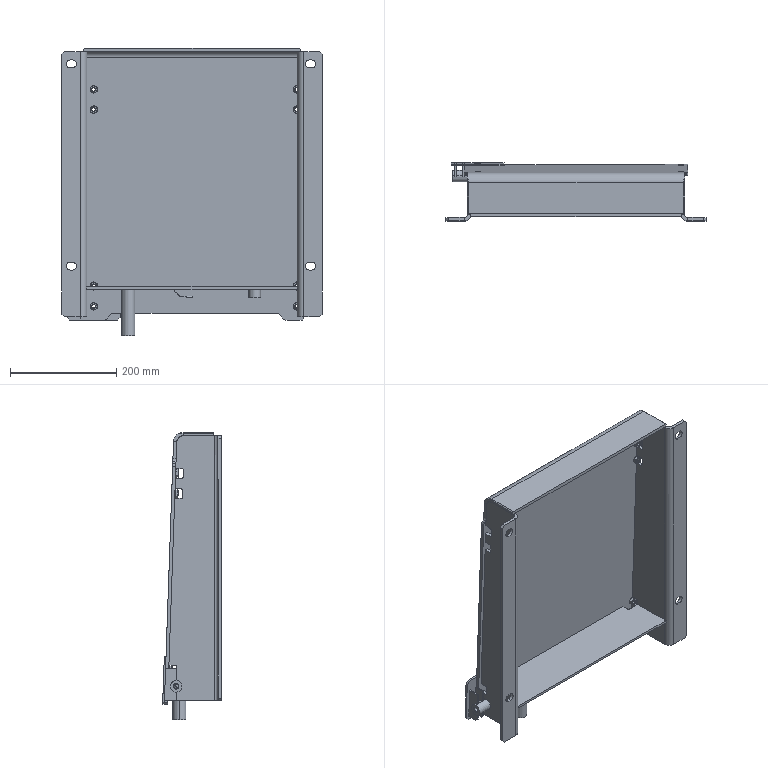Part | SolidWorks | features ReferencePattern 8, LocalLPattern 4, InContextFeatHolder 2, Cut 1 | 20 solids | 524 faces | box 490 x 110.428 x 539.749 mm | volume 2418391 mm3 | plane 279 | cylinder 125 | cone 112 | spline 8 | commonest cylinder face diameters 10 x22 6 x19 6.8 x16 15 x12 20 x10 8.5 x6